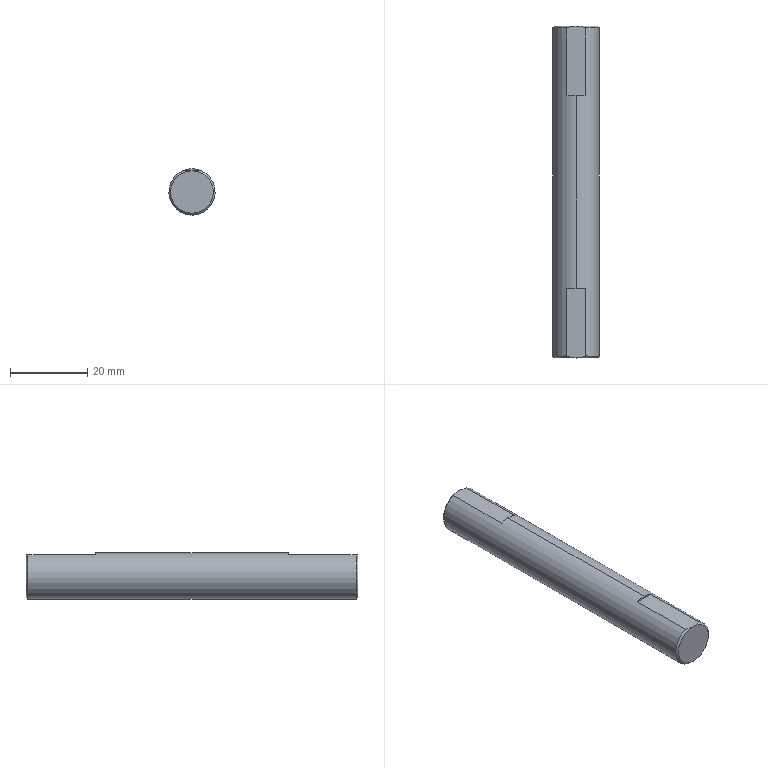Part | STEP file | ND25021-01-JDKM-18-GJ | 1 solid | 12 faces | box 12 x 86 x 12 mm | volume 9660 mm3 | plane 6 | cone 4 | cylinder 2 | commonest cylinder face diameters 12 x2
STEP:
#1=CARTESIAN_POINT('',(0.,0.,0.));
#2=DIRECTION('',(0.,0.,1.));
#3=DIRECTION('',(1.,0.,0.));
#4=AXIS2_PLACEMENT_3D('',#1,#2,#3);
#5=CARTESIAN_POINT('',(0.,-43.,-5.5));
#6=VERTEX_POINT('',#5);
#7=CARTESIAN_POINT('',(0.,-43.,5.5));
#8=VERTEX_POINT('',#7);
#9=CARTESIAN_POINT('',(0.,-43.,0.));
#10=DIRECTION('',(0.,-1.,0.));
#11=DIRECTION('',(0.,0.,1.));
#12=AXIS2_PLACEMENT_3D('',#9,#10,#11);
#13=CIRCLE('',#12,5.5);
#14=CARTESIAN_POINT('',(0.,-42.5,0.));
#15=DIRECTION('',(0.,1.,0.));
#16=DIRECTION('',(0.,0.,1.));
#17=AXIS2_PLACEMENT_3D('',#14,#15,#16);
#18=CONICAL_SURFACE('',#17,6.,0.7854);
#19=CARTESIAN_POINT('',(6.283,-0.5));
#20=DIRECTION('',(-1.,0.));
#21=VECTOR('',#20,1.);
#22=LINE('',#19,#21);
#23=(GEOMETRIC_REPRESENTATION_CONTEXT(2)PARAMETRIC_REPRESENTATION_CONTEXT()REPRESENTATION_CONTEXT('',''));
#24=DEFINITIONAL_REPRESENTATION('',(#22),#23);
#25=PCURVE('',#18,#24);
#26=CARTESIAN_POINT('',(0.,-43.,0.));
#27=DIRECTION('',(0.,1.,0.));
#28=DIRECTION('',(0.,0.,1.));
#29=AXIS2_PLACEMENT_3D('',#26,#27,#28);
#30=PLANE('',#29);
#31=CARTESIAN_POINT('',(5.5,0.));
#32=CARTESIAN_POINT('',(5.5,-9.526));
#33=CARTESIAN_POINT('',(-2.75,-4.763));
#34=CARTESIAN_POINT('',(-11.,0.));
#35=CARTESIAN_POINT('',(-2.75,4.763));
#36=CARTESIAN_POINT('',(5.5,9.526));
#37=CARTESIAN_POINT('',(5.5,0.));
#38=(BOUNDED_CURVE()B_SPLINE_CURVE(2,(#31,#32,#33,#34,#35,#36,#37),.UNSPECIFIED.,.T.,.F.)B_SPLINE_CURVE_WITH_KNOTS((1,2,2,2,2,1),(-2.094,0.,2.094,4.189,6.283,8.378),.UNSPECIFIED.)CURVE()GEOMETRIC_REPRESENTATION_ITEM()RATIONAL_B_SPLINE_CURVE((1.,0.5,1.,0.5,1.,0.5,1.))REPRESENTATION_ITEM(''));
#39=(GEOMETRIC_REPRESENTATION_CONTEXT(2)PARAMETRIC_REPRESENTATION_CONTEXT()REPRESENTATION_CONTEXT('',''));
#40=DEFINITIONAL_REPRESENTATION('',(#38),#39);
#41=PCURVE('',#30,#40);
#42=SURFACE_CURVE('',#13,(#25,#41),.PCURVE_S1.);
#43=EDGE_CURVE('',#6,#8,#42,.T.);
#44=ORIENTED_EDGE('',*,*,#43,.F.);
#45=CARTESIAN_POINT('',(0.,-42.5,-6.));
#46=VERTEX_POINT('',#45);
#47=CARTESIAN_POINT('',(0.,-42.5,-6.));
#48=DIRECTION('',(0.,0.7071,-0.7071));
#49=VECTOR('',#48,1.);
#50=LINE('',#47,#49);
#51=CARTESIAN_POINT('',(3.142,0.));
#52=DIRECTION('',(0.,1.));
#53=VECTOR('',#52,1.);
#54=LINE('',#51,#53);
#55=(GEOMETRIC_REPRESENTATION_CONTEXT(2)PARAMETRIC_REPRESENTATION_CONTEXT()REPRESENTATION_CONTEXT('',''));
#56=DEFINITIONAL_REPRESENTATION('',(#54),#55);
#57=PCURVE('',#18,#56);
#58=CARTESIAN_POINT('',(0.,-42.5,0.));
#59=DIRECTION('',(0.,1.,0.));
#60=DIRECTION('',(0.,0.,1.));
#61=AXIS2_PLACEMENT_3D('',#58,#59,#60);
#62=CONICAL_SURFACE('',#61,6.,0.7854);
#63=CARTESIAN_POINT('',(3.142,0.));
#64=DIRECTION('',(0.,1.));
#65=VECTOR('',#64,1.);
#66=LINE('',#63,#65);
#67=(GEOMETRIC_REPRESENTATION_CONTEXT(2)PARAMETRIC_REPRESENTATION_CONTEXT()REPRESENTATION_CONTEXT('',''));
#68=DEFINITIONAL_REPRESENTATION('',(#66),#67);
#69=PCURVE('',#62,#68);
#70=SURFACE_CURVE('',#50,(#57,#69),.PCURVE_S1.);
#71=EDGE_CURVE('',#6,#46,#70,.T.);
#72=ORIENTED_EDGE('',*,*,#71,.T.);
#73=CARTESIAN_POINT('',(2.398,-42.5,5.5));
#74=VERTEX_POINT('',#73);
#75=CARTESIAN_POINT('',(0.,-42.5,0.));
#76=DIRECTION('',(0.,1.,0.));
#77=DIRECTION('',(0.,0.,1.));
#78=AXIS2_PLACEMENT_3D('',#75,#76,#77);
#79=CIRCLE('',#78,6.);
#80=CARTESIAN_POINT('',(0.,0.));
#81=DIRECTION('',(1.,0.));
#82=VECTOR('',#81,1.);
#83=LINE('',#80,#82);
#84=(GEOMETRIC_REPRESENTATION_CONTEXT(2)PARAMETRIC_REPRESENTATION_CONTEXT()REPRESENTATION_CONTEXT('',''));
#85=DEFINITIONAL_REPRESENTATION('',(#83),#84);
#86=PCURVE('',#18,#85);
#87=CARTESIAN_POINT('',(0.,43.,0.));
#88=DIRECTION('',(0.,-1.,0.));
#89=DIRECTION('',(0.,0.,-1.));
#90=AXIS2_PLACEMENT_3D('',#87,#88,#89);
#91=CYLINDRICAL_SURFACE('',#90,6.);
#92=CARTESIAN_POINT('',(3.142,85.5));
#93=DIRECTION('',(-1.,0.));
#94=VECTOR('',#93,1.);
#95=LINE('',#92,#94);
#96=(GEOMETRIC_REPRESENTATION_CONTEXT(2)PARAMETRIC_REPRESENTATION_CONTEXT()REPRESENTATION_CONTEXT('',''));
#97=DEFINITIONAL_REPRESENTATION('',(#95),#96);
#98=PCURVE('',#91,#97);
#99=SURFACE_CURVE('',#79,(#86,#98),.PCURVE_S1.);
#100=EDGE_CURVE('',#74,#46,#99,.T.);
#101=ORIENTED_EDGE('',*,*,#100,.F.);
#102=CARTESIAN_POINT('',(0.,-43.,5.5));
#103=CARTESIAN_POINT('',(0.4145,-43.,5.5));
#104=CARTESIAN_POINT('',(0.8208,-42.953,5.5));
#105=CARTESIAN_POINT('',(1.62,-42.78,5.5));
#106=CARTESIAN_POINT('',(2.014,-42.653,5.5));
#107=CARTESIAN_POINT('',(2.398,-42.5,5.5));
#108=B_SPLINE_CURVE_WITH_KNOTS('',3,(#102,#103,#104,#105,#106,#107),.UNSPECIFIED.,.F.,.F.,(4,2,4),(0.,0.001225,0.00245),.UNSPECIFIED.);
#109=CARTESIAN_POINT('',(0.,-0.5));
#110=CARTESIAN_POINT('',(0.006852,-0.5));
#111=CARTESIAN_POINT('',(0.02053,-0.4992));
#112=CARTESIAN_POINT('',(0.04096,-0.4958));
#113=CARTESIAN_POINT('',(0.06128,-0.49));
#114=CARTESIAN_POINT('',(0.08148,-0.482));
#115=CARTESIAN_POINT('',(0.1015,-0.4719));
#116=CARTESIAN_POINT('',(0.1215,-0.4595));
#117=CARTESIAN_POINT('',(0.1412,-0.445));
#118=CARTESIAN_POINT('',(0.1608,-0.4285));
#119=CARTESIAN_POINT('',(0.1802,-0.4098));
#120=CARTESIAN_POINT('',(0.1994,-0.3892));
#121=CARTESIAN_POINT('',(0.2184,-0.3666));
#122=CARTESIAN_POINT('',(0.2372,-0.342));
#123=CARTESIAN_POINT('',(0.2557,-0.3155));
#124=CARTESIAN_POINT('',(0.274,-0.2871));
#125=CARTESIAN_POINT('',(0.2921,-0.257));
#126=CARTESIAN_POINT('',(0.31,-0.2251));
#127=CARTESIAN_POINT('',(0.3276,-0.1915));
#128=CARTESIAN_POINT('',(0.3449,-0.1563));
#129=CARTESIAN_POINT('',(0.3619,-0.1195));
#130=CARTESIAN_POINT('',(0.3786,-0.08115));
#131=CARTESIAN_POINT('',(0.395,-0.04138));
#132=CARTESIAN_POINT('',(0.4058,-0.01394));
#133=CARTESIAN_POINT('',(0.4111,0.));
#134=B_SPLINE_CURVE_WITH_KNOTS('',3,(#109,#110,#111,#112,#113,#114,#115,#116,#117,#118,#119,#120,#121,#122,#123,#124,#125,#126,#127,#128,#129,#130,#131,#132,#133),.UNSPECIFIED.,.F.,.F.,(4,1,1,1,1,1,1,1,1,1,1,1,1,1,1,1,1,1,1,1,1,1,4),(0.,0.0001114,0.0002228,0.0003341,0.0004455,0.0005569,0.0006683,0.0007797,0.0008911,0.001002,0.001114,0.001225,0.001337,0.001448,0.001559,0.001671,0.001782,0.001894,0.002005,0.002116,0.002228,0.002339,0.00245),.QUASI_UNIFORM_KNOTS.);
#135=(GEOMETRIC_REPRESENTATION_CONTEXT(2)PARAMETRIC_REPRESENTATION_CONTEXT()REPRESENTATION_CONTEXT('',''));
#136=DEFINITIONAL_REPRESENTATION('',(#134),#135);
#137=PCURVE('',#18,#136);
#138=CARTESIAN_POINT('',(-2.398,-25.,5.5));
#139=DIRECTION('',(0.,0.,-1.));
#140=DIRECTION('',(-1.,0.,0.));
#141=AXIS2_PLACEMENT_3D('',#138,#139,#140);
#142=PLANE('',#141);
#143=CARTESIAN_POINT('',(-2.398,-18.));
#144=CARTESIAN_POINT('',(-2.812,-18.));
#145=CARTESIAN_POINT('',(-3.219,-17.953));
#146=CARTESIAN_POINT('',(-4.018,-17.78));
#147=CARTESIAN_POINT('',(-4.412,-17.653));
#148=CARTESIAN_POINT('',(-4.796,-17.5));
#149=B_SPLINE_CURVE_WITH_KNOTS('',3,(#143,#144,#145,#146,#147,#148),.UNSPECIFIED.,.F.,.F.,(4,2,4),(0.,0.001225,0.00245),.UNSPECIFIED.);
#150=(GEOMETRIC_REPRESENTATION_CONTEXT(2)PARAMETRIC_REPRESENTATION_CONTEXT()REPRESENTATION_CONTEXT('',''));
#151=DEFINITIONAL_REPRESENTATION('',(#149),#150);
#152=PCURVE('',#142,#151);
#153=SURFACE_CURVE('',#108,(#137,#152),.PCURVE_S1.);
#154=EDGE_CURVE('',#8,#74,#153,.T.);
#155=ORIENTED_EDGE('',*,*,#154,.F.);
#156=EDGE_LOOP('',(#44,#72,#101,#155));
#157=FACE_BOUND('',#156,.T.);
#158=ADVANCED_FACE('',(#157),#18,.T.);
#159=CARTESIAN_POINT('',(0.,43.,-5.5));
#160=VERTEX_POINT('',#159);
#161=CARTESIAN_POINT('',(0.,43.,5.5));
#162=VERTEX_POINT('',#161);
#163=CARTESIAN_POINT('',(0.,43.,0.));
#164=DIRECTION('',(0.,1.,0.));
#165=DIRECTION('',(0.,0.,1.));
#166=AXIS2_PLACEMENT_3D('',#163,#164,#165);
#167=CIRCLE('',#166,5.5);
#168=CARTESIAN_POINT('',(0.,43.,0.));
#169=DIRECTION('',(0.,-1.,0.));
#170=DIRECTION('',(0.,0.,-1.));
#171=AXIS2_PLACEMENT_3D('',#168,#169,#170);
#172=CONICAL_SURFACE('',#171,5.5,0.7854);
#173=CARTESIAN_POINT('',(9.425,0.));
#174=DIRECTION('',(-1.,0.));
#175=VECTOR('',#174,1.);
#176=LINE('',#173,#175);
#177=(GEOMETRIC_REPRESENTATION_CONTEXT(2)PARAMETRIC_REPRESENTATION_CONTEXT()REPRESENTATION_CONTEXT('',''));
#178=DEFINITIONAL_REPRESENTATION('',(#176),#177);
#179=PCURVE('',#172,#178);
#180=CARTESIAN_POINT('',(0.,43.,0.));
#181=DIRECTION('',(0.,1.,0.));
#182=DIRECTION('',(0.,0.,1.));
#183=AXIS2_PLACEMENT_3D('',#180,#181,#182);
#184=PLANE('',#183);
#185=CARTESIAN_POINT('',(0.,0.));
#186=DIRECTION('',(1.,0.));
#187=AXIS2_PLACEMENT_2D('',#185,#186);
#188=CIRCLE('',#187,5.5);
#189=(GEOMETRIC_REPRESENTATION_CONTEXT(2)PARAMETRIC_REPRESENTATION_CONTEXT()REPRESENTATION_CONTEXT('',''));
#190=DEFINITIONAL_REPRESENTATION('',(#188),#189);
#191=PCURVE('',#184,#190);
#192=SURFACE_CURVE('',#167,(#179,#191),.PCURVE_S1.);
#193=EDGE_CURVE('',#160,#162,#192,.T.);
#194=ORIENTED_EDGE('',*,*,#193,.F.);
#195=CARTESIAN_POINT('',(0.,42.5,-6.));
#196=VERTEX_POINT('',#195);
#197=CARTESIAN_POINT('',(0.,43.,-5.5));
#198=DIRECTION('',(0.,-0.7071,-0.7071));
#199=VECTOR('',#198,1.);
#200=LINE('',#197,#199);
#201=CARTESIAN_POINT('',(6.283,0.));
#202=DIRECTION('',(0.,1.));
#203=VECTOR('',#202,1.);
#204=LINE('',#201,#203);
#205=(GEOMETRIC_REPRESENTATION_CONTEXT(2)PARAMETRIC_REPRESENTATION_CONTEXT()REPRESENTATION_CONTEXT('',''));
#206=DEFINITIONAL_REPRESENTATION('',(#204),#205);
#207=PCURVE('',#172,#206);
#208=CARTESIAN_POINT('',(0.,43.,0.));
#209=DIRECTION('',(0.,-1.,0.));
#210=DIRECTION('',(0.,0.,-1.));
#211=AXIS2_PLACEMENT_3D('',#208,#209,#210);
#212=CONICAL_SURFACE('',#211,5.5,0.7854);
#213=CARTESIAN_POINT('',(0.,0.));
#214=DIRECTION('',(0.,1.));
#215=VECTOR('',#214,1.);
#216=LINE('',#213,#215);
#217=(GEOMETRIC_REPRESENTATION_CONTEXT(2)PARAMETRIC_REPRESENTATION_CONTEXT()REPRESENTATION_CONTEXT('',''));
#218=DEFINITIONAL_REPRESENTATION('',(#216),#217);
#219=PCURVE('',#212,#218);
#220=SURFACE_CURVE('',#200,(#207,#219),.PCURVE_S1.);
#221=EDGE_CURVE('',#160,#196,#220,.T.);
#222=ORIENTED_EDGE('',*,*,#221,.T.);
#223=CARTESIAN_POINT('',(-2.398,42.5,5.5));
#224=VERTEX_POINT('',#223);
#225=CARTESIAN_POINT('',(0.,42.5,0.));
#226=DIRECTION('',(0.,-1.,0.));
#227=DIRECTION('',(0.,0.,1.));
#228=AXIS2_PLACEMENT_3D('',#225,#226,#227);
#229=CIRCLE('',#228,6.);
#230=CARTESIAN_POINT('',(3.142,0.5));
#231=DIRECTION('',(1.,0.));
#232=VECTOR('',#231,1.);
#233=LINE('',#230,#232);
#234=(GEOMETRIC_REPRESENTATION_CONTEXT(2)PARAMETRIC_REPRESENTATION_CONTEXT()REPRESENTATION_CONTEXT('',''));
#235=DEFINITIONAL_REPRESENTATION('',(#233),#234);
#236=PCURVE('',#172,#235);
#237=CARTESIAN_POINT('',(0.,43.,0.));
#238=DIRECTION('',(0.,-1.,0.));
#239=DIRECTION('',(0.,0.,-1.));
#240=AXIS2_PLACEMENT_3D('',#237,#238,#239);
#241=CYLINDRICAL_SURFACE('',#240,6.);
#242=CARTESIAN_POINT('',(3.142,0.5));
#243=DIRECTION('',(1.,0.));
#244=VECTOR('',#243,1.);
#245=LINE('',#242,#244);
#246=(GEOMETRIC_REPRESENTATION_CONTEXT(2)PARAMETRIC_REPRESENTATION_CONTEXT()REPRESENTATION_CONTEXT('',''));
#247=DEFINITIONAL_REPRESENTATION('',(#245),#246);
#248=PCURVE('',#241,#247);
#249=SURFACE_CURVE('',#229,(#236,#248),.PCURVE_S1.);
#250=EDGE_CURVE('',#224,#196,#249,.T.);
#251=ORIENTED_EDGE('',*,*,#250,.F.);
#252=CARTESIAN_POINT('',(0.,43.,5.5));
#253=CARTESIAN_POINT('',(-0.4145,43.,5.5));
#254=CARTESIAN_POINT('',(-0.8208,42.953,5.5));
#255=CARTESIAN_POINT('',(-1.62,42.78,5.5));
#256=CARTESIAN_POINT('',(-2.014,42.653,5.5));
#257=CARTESIAN_POINT('',(-2.398,42.5,5.5));
#258=B_SPLINE_CURVE_WITH_KNOTS('',3,(#252,#253,#254,#255,#256,#257),.UNSPECIFIED.,.F.,.F.,(4,2,4),(0.,0.001225,0.00245),.UNSPECIFIED.);
#259=CARTESIAN_POINT('',(3.142,0.));
#260=CARTESIAN_POINT('',(3.148,-0.000000092));
#261=CARTESIAN_POINT('',(3.162,0.0007776));
#262=CARTESIAN_POINT('',(3.183,0.004246));
#263=CARTESIAN_POINT('',(3.203,0.009984));
#264=CARTESIAN_POINT('',(3.223,0.01796));
#265=CARTESIAN_POINT('',(3.243,0.02814));
#266=CARTESIAN_POINT('',(3.263,0.04048));
#267=CARTESIAN_POINT('',(3.283,0.05496));
#268=CARTESIAN_POINT('',(3.302,0.07153));
#269=CARTESIAN_POINT('',(3.322,0.09015));
#270=CARTESIAN_POINT('',(3.341,0.1108));
#271=CARTESIAN_POINT('',(3.36,0.1334));
#272=CARTESIAN_POINT('',(3.379,0.158));
#273=CARTESIAN_POINT('',(3.397,0.1845));
#274=CARTESIAN_POINT('',(3.416,0.2129));
#275=CARTESIAN_POINT('',(3.434,0.243));
#276=CARTESIAN_POINT('',(3.452,0.2749));
#277=CARTESIAN_POINT('',(3.469,0.3085));
#278=CARTESIAN_POINT('',(3.486,0.3437));
#279=CARTESIAN_POINT('',(3.503,0.3805));
#280=CARTESIAN_POINT('',(3.52,0.4189));
#281=CARTESIAN_POINT('',(3.537,0.4586));
#282=CARTESIAN_POINT('',(3.547,0.4861));
#283=CARTESIAN_POINT('',(3.553,0.5));
#284=B_SPLINE_CURVE_WITH_KNOTS('',3,(#259,#260,#261,#262,#263,#264,#265,#266,#267,#268,#269,#270,#271,#272,#273,#274,#275,#276,#277,#278,#279,#280,#281,#282,#283),.UNSPECIFIED.,.F.,.F.,(4,1,1,1,1,1,1,1,1,1,1,1,1,1,1,1,1,1,1,1,1,1,4),(0.,0.0001114,0.0002228,0.0003341,0.0004455,0.0005569,0.0006683,0.0007797,0.0008911,0.001002,0.001114,0.001225,0.001337,0.001448,0.001559,0.001671,0.001782,0.001894,0.002005,0.002116,0.002228,0.002339,0.00245),.QUASI_UNIFORM_KNOTS.);
#285=(GEOMETRIC_REPRESENTATION_CONTEXT(2)PARAMETRIC_REPRESENTATION_CONTEXT()REPRESENTATION_CONTEXT('',''));
#286=DEFINITIONAL_REPRESENTATION('',(#284),#285);
#287=PCURVE('',#172,#286);
#288=CARTESIAN_POINT('',(-2.398,25.,5.5));
#289=DIRECTION('',(0.,0.,1.));
#290=DIRECTION('',(1.,0.,0.));
#291=AXIS2_PLACEMENT_3D('',#288,#289,#290);
#292=PLANE('',#291);
#293=CARTESIAN_POINT('',(2.398,18.));
#294=CARTESIAN_POINT('',(1.983,18.));
#295=CARTESIAN_POINT('',(1.577,17.953));
#296=CARTESIAN_POINT('',(0.7781,17.78));
#297=CARTESIAN_POINT('',(0.3837,17.653));
#298=CARTESIAN_POINT('',(0.,17.5));
#299=B_SPLINE_CURVE_WITH_KNOTS('',3,(#293,#294,#295,#296,#297,#298),.UNSPECIFIED.,.F.,.F.,(4,2,4),(0.,0.001225,0.00245),.UNSPECIFIED.);
#300=(GEOMETRIC_REPRESENTATION_CONTEXT(2)PARAMETRIC_REPRESENTATION_CONTEXT()REPRESENTATION_CONTEXT('',''));
#301=DEFINITIONAL_REPRESENTATION('',(#299),#300);
#302=PCURVE('',#292,#301);
#303=SURFACE_CURVE('',#258,(#287,#302),.PCURVE_S1.);
#304=EDGE_CURVE('',#162,#224,#303,.T.);
#305=ORIENTED_EDGE('',*,*,#304,.F.);
#306=EDGE_LOOP('',(#194,#222,#251,#305));
#307=FACE_BOUND('',#306,.T.);
#308=ADVANCED_FACE('',(#307),#172,.T.);
#309=CARTESIAN_POINT('',(0.,25.,6.));
#310=VERTEX_POINT('',#309);
#311=CARTESIAN_POINT('',(2.398,25.,5.5));
#312=VERTEX_POINT('',#311);
#313=CARTESIAN_POINT('',(0.,25.,0.));
#314=DIRECTION('',(0.,1.,0.));
#315=DIRECTION('',(0.,0.,1.));
#316=AXIS2_PLACEMENT_3D('',#313,#314,#315);
#317=CIRCLE('',#316,6.);
#318=CARTESIAN_POINT('',(3.142,18.));
#319=DIRECTION('',(-1.,0.));
#320=VECTOR('',#319,1.);
#321=LINE('',#318,#320);
#322=(GEOMETRIC_REPRESENTATION_CONTEXT(2)PARAMETRIC_REPRESENTATION_CONTEXT()REPRESENTATION_CONTEXT('',''));
#323=DEFINITIONAL_REPRESENTATION('',(#321),#322);
#324=PCURVE('',#91,#323);
#325=CARTESIAN_POINT('',(0.,25.,0.));
#326=DIRECTION('',(0.,1.,0.));
#327=DIRECTION('',(0.,0.,-1.));
#328=AXIS2_PLACEMENT_3D('',#325,#326,#327);
#329=PLANE('',#328);
#330=CARTESIAN_POINT('',(0.,0.));
#331=DIRECTION('',(-1.,0.));
#332=AXIS2_PLACEMENT_2D('',#330,#331);
#333=CIRCLE('',#332,6.);
#334=(GEOMETRIC_REPRESENTATION_CONTEXT(2)PARAMETRIC_REPRESENTATION_CONTEXT()REPRESENTATION_CONTEXT('',''));
#335=DEFINITIONAL_REPRESENTATION('',(#333),#334);
#336=PCURVE('',#329,#335);
#337=SURFACE_CURVE('',#317,(#324,#336),.PCURVE_S1.);
#338=EDGE_CURVE('',#310,#312,#337,.T.);
#339=ORIENTED_EDGE('',*,*,#338,.F.);
#340=CARTESIAN_POINT('',(0.,-25.,6.));
#341=VERTEX_POINT('',#340);
#342=CARTESIAN_POINT('',(0.,43.,6.));
#343=DIRECTION('',(0.,-1.,0.));
#344=VECTOR('',#343,1.);
#345=LINE('',#342,#344);
#346=CARTESIAN_POINT('',(3.142,0.));
#347=DIRECTION('',(0.,1.));
#348=VECTOR('',#347,1.);
#349=LINE('',#346,#348);
#350=(GEOMETRIC_REPRESENTATION_CONTEXT(2)PARAMETRIC_REPRESENTATION_CONTEXT()REPRESENTATION_CONTEXT('',''));
#351=DEFINITIONAL_REPRESENTATION('',(#349),#350);
#352=PCURVE('',#91,#351);
#353=CARTESIAN_POINT('',(3.142,0.));
#354=DIRECTION('',(0.,1.));
#355=VECTOR('',#354,1.);
#356=LINE('',#353,#355);
#357=(GEOMETRIC_REPRESENTATION_CONTEXT(2)PARAMETRIC_REPRESENTATION_CONTEXT()REPRESENTATION_CONTEXT('',''));
#358=DEFINITIONAL_REPRESENTATION('',(#356),#357);
#359=PCURVE('',#241,#358);
#360=SURFACE_CURVE('',#345,(#352,#359),.PCURVE_S1.);
#361=EDGE_CURVE('',#310,#341,#360,.T.);
#362=ORIENTED_EDGE('',*,*,#361,.T.);
#363=CARTESIAN_POINT('',(2.398,-25.,5.5));
#364=VERTEX_POINT('',#363);
#365=CARTESIAN_POINT('',(0.,-25.,0.));
#366=DIRECTION('',(0.,-1.,0.));
#367=DIRECTION('',(0.,0.,-1.));
#368=AXIS2_PLACEMENT_3D('',#365,#366,#367);
#369=CIRCLE('',#368,6.);
#370=CARTESIAN_POINT('',(0.,68.));
#371=DIRECTION('',(1.,0.));
#372=VECTOR('',#371,1.);
#373=LINE('',#370,#372);
#374=(GEOMETRIC_REPRESENTATION_CONTEXT(2)PARAMETRIC_REPRESENTATION_CONTEXT()REPRESENTATION_CONTEXT('',''));
#375=DEFINITIONAL_REPRESENTATION('',(#373),#374);
#376=PCURVE('',#91,#375);
#377=CARTESIAN_POINT('',(0.,-25.,0.));
#378=DIRECTION('',(0.,-1.,0.));
#379=DIRECTION('',(0.,0.,-1.));
#380=AXIS2_PLACEMENT_3D('',#377,#378,#379);
#381=PLANE('',#380);
#382=CARTESIAN_POINT('',(0.,0.));
#383=DIRECTION('',(1.,0.));
#384=AXIS2_PLACEMENT_2D('',#382,#383);
#385=CIRCLE('',#384,6.);
#386=(GEOMETRIC_REPRESENTATION_CONTEXT(2)PARAMETRIC_REPRESENTATION_CONTEXT()REPRESENTATION_CONTEXT('',''));
#387=DEFINITIONAL_REPRESENTATION('',(#385),#386);
#388=PCURVE('',#381,#387);
#389=SURFACE_CURVE('',#369,(#376,#388),.PCURVE_S1.);
#390=EDGE_CURVE('',#364,#341,#389,.T.);
#391=ORIENTED_EDGE('',*,*,#390,.F.);
#392=CARTESIAN_POINT('',(2.398,-25.,5.5));
#393=DIRECTION('',(0.,-1.,0.));
#394=VECTOR('',#393,1.);
#395=LINE('',#392,#394);
#396=CARTESIAN_POINT('',(2.73,68.));
#397=DIRECTION('',(0.,1.));
#398=VECTOR('',#397,1.);
#399=LINE('',#396,#398);
#400=(GEOMETRIC_REPRESENTATION_CONTEXT(2)PARAMETRIC_REPRESENTATION_CONTEXT()REPRESENTATION_CONTEXT('',''));
#401=DEFINITIONAL_REPRESENTATION('',(#399),#400);
#402=PCURVE('',#91,#401);
#403=CARTESIAN_POINT('',(-4.796,0.));
#404=DIRECTION('',(0.,-1.));
#405=VECTOR('',#404,1.);
#406=LINE('',#403,#405);
#407=(GEOMETRIC_REPRESENTATION_CONTEXT(2)PARAMETRIC_REPRESENTATION_CONTEXT()REPRESENTATION_CONTEXT('',''));
#408=DEFINITIONAL_REPRESENTATION('',(#406),#407);
#409=PCURVE('',#142,#408);
#410=SURFACE_CURVE('',#395,(#402,#409),.PCURVE_S1.);
#411=EDGE_CURVE('',#364,#74,#410,.T.);
#412=ORIENTED_EDGE('',*,*,#411,.T.);
#413=ORIENTED_EDGE('',*,*,#100,.T.);
#414=CARTESIAN_POINT('',(0.,43.,-6.));
#415=DIRECTION('',(0.,-1.,0.));
#416=VECTOR('',#415,1.);
#417=LINE('',#414,#416);
#418=CARTESIAN_POINT('',(0.,0.));
#419=DIRECTION('',(0.,1.));
#420=VECTOR('',#419,1.);
#421=LINE('',#418,#420);
#422=(GEOMETRIC_REPRESENTATION_CONTEXT(2)PARAMETRIC_REPRESENTATION_CONTEXT()REPRESENTATION_CONTEXT('',''));
#423=DEFINITIONAL_REPRESENTATION('',(#421),#422);
#424=PCURVE('',#91,#423);
#425=CARTESIAN_POINT('',(6.283,0.));
#426=DIRECTION('',(0.,1.));
#427=VECTOR('',#426,1.);
#428=LINE('',#425,#427);
#429=(GEOMETRIC_REPRESENTATION_CONTEXT(2)PARAMETRIC_REPRESENTATION_CONTEXT()REPRESENTATION_CONTEXT('',''));
#430=DEFINITIONAL_REPRESENTATION('',(#428),#429);
#431=PCURVE('',#241,#430);
#432=SURFACE_CURVE('',#417,(#424,#431),.PCURVE_S1.);
#433=EDGE_CURVE('',#196,#46,#432,.T.);
#434=ORIENTED_EDGE('',*,*,#433,.F.);
#435=CARTESIAN_POINT('',(2.398,42.5,5.5));
#436=VERTEX_POINT('',#435);
#437=CARTESIAN_POINT('',(0.,42.5,0.));
#438=DIRECTION('',(0.,-1.,0.));
#439=DIRECTION('',(0.,0.,1.));
#440=AXIS2_PLACEMENT_3D('',#437,#438,#439);
#441=CIRCLE('',#440,6.);
#442=CARTESIAN_POINT('',(-3.142,0.5));
#443=DIRECTION('',(1.,0.));
#444=VECTOR('',#443,1.);
#445=LINE('',#442,#444);
#446=(GEOMETRIC_REPRESENTATION_CONTEXT(2)PARAMETRIC_REPRESENTATION_CONTEXT()REPRESENTATION_CONTEXT('',''));
#447=DEFINITIONAL_REPRESENTATION('',(#445),#446);
#448=PCURVE('',#91,#447);
#449=CARTESIAN_POINT('',(-3.142,0.5));
#450=DIRECTION('',(1.,0.));
#451=VECTOR('',#450,1.);
#452=LINE('',#449,#451);
#453=(GEOMETRIC_REPRESENTATION_CONTEXT(2)PARAMETRIC_REPRESENTATION_CONTEXT()REPRESENTATION_CONTEXT('',''));
#454=DEFINITIONAL_REPRESENTATION('',(#452),#453);
#455=PCURVE('',#212,#454);
#456=SURFACE_CURVE('',#441,(#448,#455),.PCURVE_S1.);
#457=EDGE_CURVE('',#196,#436,#456,.T.);
#458=ORIENTED_EDGE('',*,*,#457,.T.);
#459=CARTESIAN_POINT('',(2.398,25.,5.5));
#460=DIRECTION('',(0.,1.,0.));
#461=VECTOR('',#460,1.);
#462=LINE('',#459,#461);
#463=CARTESIAN_POINT('',(2.73,18.));
#464=DIRECTION('',(0.,-1.));
#465=VECTOR('',#464,1.);
#466=LINE('',#463,#465);
#467=(GEOMETRIC_REPRESENTATION_CONTEXT(2)PARAMETRIC_REPRESENTATION_CONTEXT()REPRESENTATION_CONTEXT('',''));
#468=DEFINITIONAL_REPRESENTATION('',(#466),#467);
#469=PCURVE('',#91,#468);
#470=CARTESIAN_POINT('',(4.796,0.));
#471=DIRECTION('',(0.,1.));
#472=VECTOR('',#471,1.);
#473=LINE('',#470,#472);
#474=(GEOMETRIC_REPRESENTATION_CONTEXT(2)PARAMETRIC_REPRESENTATION_CONTEXT()REPRESENTATION_CONTEXT('',''));
#475=DEFINITIONAL_REPRESENTATION('',(#473),#474);
#476=PCURVE('',#292,#475);
#477=SURFACE_CURVE('',#462,(#469,#476),.PCURVE_S1.);
#478=EDGE_CURVE('',#312,#436,#477,.T.);
#479=ORIENTED_EDGE('',*,*,#478,.F.);
#480=EDGE_LOOP('',(#339,#362,#391,#412,#413,#434,#458,#479));
#481=FACE_BOUND('',#480,.T.);
#482=ADVANCED_FACE('',(#481),#91,.T.);
#483=ORIENTED_EDGE('',*,*,#361,.F.);
#484=CARTESIAN_POINT('',(-2.398,25.,5.5));
#485=VERTEX_POINT('',#484);
#486=CARTESIAN_POINT('',(0.,25.,0.));
#487=DIRECTION('',(0.,1.,0.));
#488=DIRECTION('',(0.,0.,1.));
#489=AXIS2_PLACEMENT_3D('',#486,#487,#488);
#490=CIRCLE('',#489,6.);
#491=CARTESIAN_POINT('',(9.425,18.));
#492=DIRECTION('',(-1.,0.));
#493=VECTOR('',#492,1.);
#494=LINE('',#491,#493);
#495=(GEOMETRIC_REPRESENTATION_CONTEXT(2)PARAMETRIC_REPRESENTATION_CONTEXT()REPRESENTATION_CONTEXT('',''));
#496=DEFINITIONAL_REPRESENTATION('',(#494),#495);
#497=PCURVE('',#241,#496);
#498=CARTESIAN_POINT('',(0.,0.));
#499=DIRECTION('',(-1.,0.));
#500=AXIS2_PLACEMENT_2D('',#498,#499);
#501=CIRCLE('',#500,6.);
#502=(GEOMETRIC_REPRESENTATION_CONTEXT(2)PARAMETRIC_REPRESENTATION_CONTEXT()REPRESENTATION_CONTEXT('',''));
#503=DEFINITIONAL_REPRESENTATION('',(#501),#502);
#504=PCURVE('',#329,#503);
#505=SURFACE_CURVE('',#490,(#497,#504),.PCURVE_S1.);
#506=EDGE_CURVE('',#485,#310,#505,.T.);
#507=ORIENTED_EDGE('',*,*,#506,.F.);
#508=CARTESIAN_POINT('',(-2.398,25.,5.5));
#509=DIRECTION('',(0.,1.,0.));
#510=VECTOR('',#509,1.);
#511=LINE('',#508,#510);
#512=CARTESIAN_POINT('',(3.553,18.));
#513=DIRECTION('',(0.,-1.));
#514=VECTOR('',#513,1.);
#515=LINE('',#512,#514);
#516=(GEOMETRIC_REPRESENTATION_CONTEXT(2)PARAMETRIC_REPRESENTATION_CONTEXT()REPRESENTATION_CONTEXT('',''));
#517=DEFINITIONAL_REPRESENTATION('',(#515),#516);
#518=PCURVE('',#241,#517);
#519=CARTESIAN_POINT('',(0.,0.));
#520=DIRECTION('',(0.,1.));
#521=VECTOR('',#520,1.);
#522=LINE('',#519,#521);
#523=(GEOMETRIC_REPRESENTATION_CONTEXT(2)PARAMETRIC_REPRESENTATION_CONTEXT()REPRESENTATION_CONTEXT('',''));
#524=DEFINITIONAL_REPRESENTATION('',(#522),#523);
#525=PCURVE('',#292,#524);
#526=SURFACE_CURVE('',#511,(#518,#525),.PCURVE_S1.);
#527=EDGE_CURVE('',#485,#224,#526,.T.);
#528=ORIENTED_EDGE('',*,*,#527,.T.);
#529=ORIENTED_EDGE('',*,*,#250,.T.);
#530=ORIENTED_EDGE('',*,*,#433,.T.);
#531=CARTESIAN_POINT('',(-2.398,-42.5,5.5));
#532=VERTEX_POINT('',#531);
#533=CARTESIAN_POINT('',(0.,-42.5,0.));
#534=DIRECTION('',(0.,1.,0.));
#535=DIRECTION('',(0.,0.,1.));
#536=AXIS2_PLACEMENT_3D('',#533,#534,#535);
#537=CIRCLE('',#536,6.);
#538=CARTESIAN_POINT('',(9.425,85.5));
#539=DIRECTION('',(-1.,0.));
#540=VECTOR('',#539,1.);
#541=LINE('',#538,#540);
#542=(GEOMETRIC_REPRESENTATION_CONTEXT(2)PARAMETRIC_REPRESENTATION_CONTEXT()REPRESENTATION_CONTEXT('',''));
#543=DEFINITIONAL_REPRESENTATION('',(#541),#542);
#544=PCURVE('',#241,#543);
#545=CARTESIAN_POINT('',(0.,0.));
#546=DIRECTION('',(1.,0.));
#547=VECTOR('',#546,1.);
#548=LINE('',#545,#547);
#549=(GEOMETRIC_REPRESENTATION_CONTEXT(2)PARAMETRIC_REPRESENTATION_CONTEXT()REPRESENTATION_CONTEXT('',''));
#550=DEFINITIONAL_REPRESENTATION('',(#548),#549);
#551=PCURVE('',#62,#550);
#552=SURFACE_CURVE('',#537,(#544,#551),.PCURVE_S1.);
#553=EDGE_CURVE('',#46,#532,#552,.T.);
#554=ORIENTED_EDGE('',*,*,#553,.T.);
#555=CARTESIAN_POINT('',(-2.398,-25.,5.5));
#556=VERTEX_POINT('',#555);
#557=CARTESIAN_POINT('',(-2.398,-25.,5.5));
#558=DIRECTION('',(0.,-1.,0.));
#559=VECTOR('',#558,1.);
#560=LINE('',#557,#559);
#561=CARTESIAN_POINT('',(3.553,68.));
#562=DIRECTION('',(0.,1.));
#563=VECTOR('',#562,1.);
#564=LINE('',#561,#563);
#565=(GEOMETRIC_REPRESENTATION_CONTEXT(2)PARAMETRIC_REPRESENTATION_CONTEXT()REPRESENTATION_CONTEXT('',''));
#566=DEFINITIONAL_REPRESENTATION('',(#564),#565);
#567=PCURVE('',#241,#566);
#568=CARTESIAN_POINT('',(0.,0.));
#569=DIRECTION('',(0.,-1.));
#570=VECTOR('',#569,1.);
#571=LINE('',#568,#570);
#572=(GEOMETRIC_REPRESENTATION_CONTEXT(2)PARAMETRIC_REPRESENTATION_CONTEXT()REPRESENTATION_CONTEXT('',''));
#573=DEFINITIONAL_REPRESENTATION('',(#571),#572);
#574=PCURVE('',#142,#573);
#575=SURFACE_CURVE('',#560,(#567,#574),.PCURVE_S1.);
#576=EDGE_CURVE('',#556,#532,#575,.T.);
#577=ORIENTED_EDGE('',*,*,#576,.F.);
#578=CARTESIAN_POINT('',(0.,-25.,0.));
#579=DIRECTION('',(0.,-1.,0.));
#580=DIRECTION('',(0.,0.,-1.));
#581=AXIS2_PLACEMENT_3D('',#578,#579,#580);
#582=CIRCLE('',#581,6.);
#583=CARTESIAN_POINT('',(0.,68.));
#584=DIRECTION('',(1.,0.));
#585=VECTOR('',#584,1.);
#586=LINE('',#583,#585);
#587=(GEOMETRIC_REPRESENTATION_CONTEXT(2)PARAMETRIC_REPRESENTATION_CONTEXT()REPRESENTATION_CONTEXT('',''));
#588=DEFINITIONAL_REPRESENTATION('',(#586),#587);
#589=PCURVE('',#241,#588);
#590=CARTESIAN_POINT('',(0.,0.));
#591=DIRECTION('',(1.,0.));
#592=AXIS2_PLACEMENT_2D('',#590,#591);
#593=CIRCLE('',#592,6.);
#594=(GEOMETRIC_REPRESENTATION_CONTEXT(2)PARAMETRIC_REPRESENTATION_CONTEXT()REPRESENTATION_CONTEXT('',''));
#595=DEFINITIONAL_REPRESENTATION('',(#593),#594);
#596=PCURVE('',#381,#595);
#597=SURFACE_CURVE('',#582,(#589,#596),.PCURVE_S1.);
#598=EDGE_CURVE('',#341,#556,#597,.T.);
#599=ORIENTED_EDGE('',*,*,#598,.F.);
#600=EDGE_LOOP('',(#483,#507,#528,#529,#530,#554,#577,#599));
#601=FACE_BOUND('',#600,.T.);
#602=ADVANCED_FACE('',(#601),#241,.T.);
#603=CARTESIAN_POINT('',(0.,43.,0.));
#604=DIRECTION('',(0.,1.,0.));
#605=DIRECTION('',(0.,0.,1.));
#606=AXIS2_PLACEMENT_3D('',#603,#604,#605);
#607=CIRCLE('',#606,5.5);
#608=CARTESIAN_POINT('',(0.,0.));
#609=DIRECTION('',(1.,0.));
#610=AXIS2_PLACEMENT_2D('',#608,#609);
#611=CIRCLE('',#610,5.5);
#612=(GEOMETRIC_REPRESENTATION_CONTEXT(2)PARAMETRIC_REPRESENTATION_CONTEXT()REPRESENTATION_CONTEXT('',''));
#613=DEFINITIONAL_REPRESENTATION('',(#611),#612);
#614=PCURVE('',#184,#613);
#615=CARTESIAN_POINT('',(3.142,0.));
#616=DIRECTION('',(-1.,0.));
#617=VECTOR('',#616,1.);
#618=LINE('',#615,#617);
#619=(GEOMETRIC_REPRESENTATION_CONTEXT(2)PARAMETRIC_REPRESENTATION_CONTEXT()REPRESENTATION_CONTEXT('',''));
#620=DEFINITIONAL_REPRESENTATION('',(#618),#619);
#621=PCURVE('',#212,#620);
#622=SURFACE_CURVE('',#607,(#614,#621),.PCURVE_S1.);
#623=EDGE_CURVE('',#162,#160,#622,.T.);
#624=ORIENTED_EDGE('',*,*,#623,.T.);
#625=ORIENTED_EDGE('',*,*,#193,.T.);
#626=EDGE_LOOP('',(#624,#625));
#627=FACE_BOUND('',#626,.T.);
#628=ADVANCED_FACE('',(#627),#184,.T.);
#629=CARTESIAN_POINT('',(0.,-43.,0.));
#630=DIRECTION('',(0.,-1.,0.));
#631=DIRECTION('',(0.,0.,1.));
#632=AXIS2_PLACEMENT_3D('',#629,#630,#631);
#633=CIRCLE('',#632,5.5);
#634=CARTESIAN_POINT('',(5.5,0.));
#635=CARTESIAN_POINT('',(5.5,-9.526));
#636=CARTESIAN_POINT('',(-2.75,-4.763));
#637=CARTESIAN_POINT('',(-11.,0.));
#638=CARTESIAN_POINT('',(-2.75,4.763));
#639=CARTESIAN_POINT('',(5.5,9.526));
#640=CARTESIAN_POINT('',(5.5,0.));
#641=(BOUNDED_CURVE()B_SPLINE_CURVE(2,(#634,#635,#636,#637,#638,#639,#640),.UNSPECIFIED.,.T.,.F.)B_SPLINE_CURVE_WITH_KNOTS((1,2,2,2,2,1),(-2.094,0.,2.094,4.189,6.283,8.378),.UNSPECIFIED.)CURVE()GEOMETRIC_REPRESENTATION_ITEM()RATIONAL_B_SPLINE_CURVE((1.,0.5,1.,0.5,1.,0.5,1.))REPRESENTATION_ITEM(''));
#642=(GEOMETRIC_REPRESENTATION_CONTEXT(2)PARAMETRIC_REPRESENTATION_CONTEXT()REPRESENTATION_CONTEXT('',''));
#643=DEFINITIONAL_REPRESENTATION('',(#641),#642);
#644=PCURVE('',#30,#643);
#645=CARTESIAN_POINT('',(6.283,-0.5));
#646=DIRECTION('',(-1.,0.));
#647=VECTOR('',#646,1.);
#648=LINE('',#645,#647);
#649=(GEOMETRIC_REPRESENTATION_CONTEXT(2)PARAMETRIC_REPRESENTATION_CONTEXT()REPRESENTATION_CONTEXT('',''));
#650=DEFINITIONAL_REPRESENTATION('',(#648),#649);
#651=PCURVE('',#62,#650);
#652=SURFACE_CURVE('',#633,(#644,#651),.PCURVE_S1.);
#653=EDGE_CURVE('',#8,#6,#652,.T.);
#654=ORIENTED_EDGE('',*,*,#653,.T.);
#655=ORIENTED_EDGE('',*,*,#43,.T.);
#656=EDGE_LOOP('',(#654,#655));
#657=FACE_BOUND('',#656,.T.);
#658=ADVANCED_FACE('',(#657),#30,.F.);
#659=CARTESIAN_POINT('',(-2.398,-25.,5.5));
#660=DIRECTION('',(1.,0.,0.));
#661=VECTOR('',#660,1.);
#662=LINE('',#659,#661);
#663=CARTESIAN_POINT('',(-5.5,-2.398));
#664=DIRECTION('',(0.,1.));
#665=VECTOR('',#664,1.);
#666=LINE('',#663,#665);
#667=(GEOMETRIC_REPRESENTATION_CONTEXT(2)PARAMETRIC_REPRESENTATION_CONTEXT()REPRESENTATION_CONTEXT('',''));
#668=DEFINITIONAL_REPRESENTATION('',(#666),#667);
#669=PCURVE('',#381,#668);
#670=CARTESIAN_POINT('',(0.,0.));
#671=DIRECTION('',(-1.,0.));
#672=VECTOR('',#671,1.);
#673=LINE('',#670,#672);
#674=(GEOMETRIC_REPRESENTATION_CONTEXT(2)PARAMETRIC_REPRESENTATION_CONTEXT()REPRESENTATION_CONTEXT('',''));
#675=DEFINITIONAL_REPRESENTATION('',(#673),#674);
#676=PCURVE('',#142,#675);
#677=SURFACE_CURVE('',#662,(#669,#676),.PCURVE_S1.);
#678=EDGE_CURVE('',#556,#364,#677,.T.);
#679=ORIENTED_EDGE('',*,*,#678,.T.);
#680=ORIENTED_EDGE('',*,*,#390,.T.);
#681=ORIENTED_EDGE('',*,*,#598,.T.);
#682=EDGE_LOOP('',(#679,#680,#681));
#683=FACE_BOUND('',#682,.T.);
#684=ADVANCED_FACE('',(#683),#381,.T.);
#685=ORIENTED_EDGE('',*,*,#576,.T.);
#686=CARTESIAN_POINT('',(-2.398,-42.5,5.5));
#687=CARTESIAN_POINT('',(-1.628,-42.808,5.5));
#688=CARTESIAN_POINT('',(-0.8341,-43.,5.5));
#689=CARTESIAN_POINT('',(0.,-43.,5.5));
#690=B_SPLINE_CURVE_WITH_KNOTS('',3,(#686,#687,#688,#689),.UNSPECIFIED.,.F.,.F.,(4,4),(0.,0.002449),.PIECEWISE_BEZIER_KNOTS.);
#691=CARTESIAN_POINT('',(0.,-17.5));
#692=CARTESIAN_POINT('',(-0.7699,-17.808));
#693=CARTESIAN_POINT('',(-1.564,-18.));
#694=CARTESIAN_POINT('',(-2.398,-18.));
#695=B_SPLINE_CURVE_WITH_KNOTS('',3,(#691,#692,#693,#694),.UNSPECIFIED.,.F.,.F.,(4,4),(0.,0.002449),.PIECEWISE_BEZIER_KNOTS.);
#696=(GEOMETRIC_REPRESENTATION_CONTEXT(2)PARAMETRIC_REPRESENTATION_CONTEXT()REPRESENTATION_CONTEXT('',''));
#697=DEFINITIONAL_REPRESENTATION('',(#695),#696);
#698=PCURVE('',#142,#697);
#699=CARTESIAN_POINT('',(5.872,0.));
#700=CARTESIAN_POINT('',(5.877,-0.01399));
#701=CARTESIAN_POINT('',(5.888,-0.04148));
#702=CARTESIAN_POINT('',(5.905,-0.08126));
#703=CARTESIAN_POINT('',(5.921,-0.1195));
#704=CARTESIAN_POINT('',(5.938,-0.1562));
#705=CARTESIAN_POINT('',(5.956,-0.1913));
#706=CARTESIAN_POINT('',(5.973,-0.2248));
#707=CARTESIAN_POINT('',(5.991,-0.2566));
#708=CARTESIAN_POINT('',(6.009,-0.2866));
#709=CARTESIAN_POINT('',(6.027,-0.3148));
#710=CARTESIAN_POINT('',(6.046,-0.3413));
#711=CARTESIAN_POINT('',(6.064,-0.3658));
#712=CARTESIAN_POINT('',(6.083,-0.3885));
#713=CARTESIAN_POINT('',(6.102,-0.4092));
#714=CARTESIAN_POINT('',(6.122,-0.4279));
#715=CARTESIAN_POINT('',(6.141,-0.4446));
#716=CARTESIAN_POINT('',(6.161,-0.4591));
#717=CARTESIAN_POINT('',(6.181,-0.4716));
#718=CARTESIAN_POINT('',(6.201,-0.4818));
#719=CARTESIAN_POINT('',(6.222,-0.4899));
#720=CARTESIAN_POINT('',(6.242,-0.4957));
#721=CARTESIAN_POINT('',(6.263,-0.4992));
#722=CARTESIAN_POINT('',(6.276,-0.5));
#723=CARTESIAN_POINT('',(6.283,-0.5));
#724=B_SPLINE_CURVE_WITH_KNOTS('',3,(#699,#700,#701,#702,#703,#704,#705,#706,#707,#708,#709,#710,#711,#712,#713,#714,#715,#716,#717,#718,#719,#720,#721,#722,#723),.UNSPECIFIED.,.F.,.F.,(4,1,1,1,1,1,1,1,1,1,1,1,1,1,1,1,1,1,1,1,1,1,4),(0.,0.0001113,0.0002227,0.000334,0.0004454,0.0005567,0.000668,0.0007794,0.0008907,0.001002,0.001113,0.001225,0.001336,0.001447,0.001559,0.00167,0.001781,0.001893,0.002004,0.002115,0.002227,0.002338,0.002449),.QUASI_UNIFORM_KNOTS.);
#725=(GEOMETRIC_REPRESENTATION_CONTEXT(2)PARAMETRIC_REPRESENTATION_CONTEXT()REPRESENTATION_CONTEXT('',''));
#726=DEFINITIONAL_REPRESENTATION('',(#724),#725);
#727=PCURVE('',#62,#726);
#728=SURFACE_CURVE('',#690,(#698,#727),.PCURVE_S1.);
#729=EDGE_CURVE('',#532,#8,#728,.T.);
#730=ORIENTED_EDGE('',*,*,#729,.T.);
#731=ORIENTED_EDGE('',*,*,#154,.T.);
#732=ORIENTED_EDGE('',*,*,#411,.F.);
#733=ORIENTED_EDGE('',*,*,#678,.F.);
#734=EDGE_LOOP('',(#685,#730,#731,#732,#733));
#735=FACE_BOUND('',#734,.T.);
#736=ADVANCED_FACE('',(#735),#142,.F.);
#737=ORIENTED_EDGE('',*,*,#506,.T.);
#738=ORIENTED_EDGE('',*,*,#338,.T.);
#739=CARTESIAN_POINT('',(-2.398,25.,5.5));
#740=DIRECTION('',(1.,0.,0.));
#741=VECTOR('',#740,1.);
#742=LINE('',#739,#741);
#743=CARTESIAN_POINT('',(-5.5,2.398));
#744=DIRECTION('',(0.,-1.));
#745=VECTOR('',#744,1.);
#746=LINE('',#743,#745);
#747=(GEOMETRIC_REPRESENTATION_CONTEXT(2)PARAMETRIC_REPRESENTATION_CONTEXT()REPRESENTATION_CONTEXT('',''));
#748=DEFINITIONAL_REPRESENTATION('',(#746),#747);
#749=PCURVE('',#329,#748);
#750=CARTESIAN_POINT('',(0.,0.));
#751=DIRECTION('',(1.,0.));
#752=VECTOR('',#751,1.);
#753=LINE('',#750,#752);
#754=(GEOMETRIC_REPRESENTATION_CONTEXT(2)PARAMETRIC_REPRESENTATION_CONTEXT()REPRESENTATION_CONTEXT('',''));
#755=DEFINITIONAL_REPRESENTATION('',(#753),#754);
#756=PCURVE('',#292,#755);
#757=SURFACE_CURVE('',#742,(#749,#756),.PCURVE_S1.);
#758=EDGE_CURVE('',#485,#312,#757,.T.);
#759=ORIENTED_EDGE('',*,*,#758,.F.);
#760=EDGE_LOOP('',(#737,#738,#759));
#761=FACE_BOUND('',#760,.T.);
#762=ADVANCED_FACE('',(#761),#329,.T.);
#763=CARTESIAN_POINT('',(2.398,42.5,5.5));
#764=CARTESIAN_POINT('',(1.628,42.808,5.5));
#765=CARTESIAN_POINT('',(0.8341,43.,5.5));
#766=CARTESIAN_POINT('',(0.,43.,5.5));
#767=B_SPLINE_CURVE_WITH_KNOTS('',3,(#763,#764,#765,#766),.UNSPECIFIED.,.F.,.F.,(4,4),(0.,0.002449),.PIECEWISE_BEZIER_KNOTS.);
#768=CARTESIAN_POINT('',(4.796,17.5));
#769=CARTESIAN_POINT('',(4.026,17.808));
#770=CARTESIAN_POINT('',(3.232,18.));
#771=CARTESIAN_POINT('',(2.398,18.));
#772=B_SPLINE_CURVE_WITH_KNOTS('',3,(#768,#769,#770,#771),.UNSPECIFIED.,.F.,.F.,(4,4),(0.,0.002449),.PIECEWISE_BEZIER_KNOTS.);
#773=(GEOMETRIC_REPRESENTATION_CONTEXT(2)PARAMETRIC_REPRESENTATION_CONTEXT()REPRESENTATION_CONTEXT('',''));
#774=DEFINITIONAL_REPRESENTATION('',(#772),#773);
#775=PCURVE('',#292,#774);
#776=CARTESIAN_POINT('',(2.73,0.5));
#777=CARTESIAN_POINT('',(2.736,0.486));
#778=CARTESIAN_POINT('',(2.747,0.4585));
#779=CARTESIAN_POINT('',(2.763,0.4187));
#780=CARTESIAN_POINT('',(2.78,0.3805));
#781=CARTESIAN_POINT('',(2.797,0.3438));
#782=CARTESIAN_POINT('',(2.814,0.3087));
#783=CARTESIAN_POINT('',(2.831,0.2752));
#784=CARTESIAN_POINT('',(2.849,0.2434));
#785=CARTESIAN_POINT('',(2.867,0.2134));
#786=CARTESIAN_POINT('',(2.886,0.1852));
#787=CARTESIAN_POINT('',(2.904,0.1587));
#788=CARTESIAN_POINT('',(2.923,0.1342));
#789=CARTESIAN_POINT('',(2.942,0.1115));
#790=CARTESIAN_POINT('',(2.961,0.0908));
#791=CARTESIAN_POINT('',(2.98,0.07211));
#792=CARTESIAN_POINT('',(3.,0.05545));
#793=CARTESIAN_POINT('',(3.02,0.04088));
#794=CARTESIAN_POINT('',(3.04,0.02844));
#795=CARTESIAN_POINT('',(3.06,0.01817));
#796=CARTESIAN_POINT('',(3.08,0.01011));
#797=CARTESIAN_POINT('',(3.1,0.004304));
#798=CARTESIAN_POINT('',(3.121,0.0007894));
#799=CARTESIAN_POINT('',(3.135,-0.000000082));
#800=CARTESIAN_POINT('',(3.142,0.));
#801=B_SPLINE_CURVE_WITH_KNOTS('',3,(#776,#777,#778,#779,#780,#781,#782,#783,#784,#785,#786,#787,#788,#789,#790,#791,#792,#793,#794,#795,#796,#797,#798,#799,#800),.UNSPECIFIED.,.F.,.F.,(4,1,1,1,1,1,1,1,1,1,1,1,1,1,1,1,1,1,1,1,1,1,4),(0.,0.0001113,0.0002227,0.000334,0.0004454,0.0005567,0.000668,0.0007794,0.0008907,0.001002,0.001113,0.001225,0.001336,0.001447,0.001559,0.00167,0.001781,0.001893,0.002004,0.002115,0.002227,0.002338,0.002449),.QUASI_UNIFORM_KNOTS.);
#802=(GEOMETRIC_REPRESENTATION_CONTEXT(2)PARAMETRIC_REPRESENTATION_CONTEXT()REPRESENTATION_CONTEXT('',''));
#803=DEFINITIONAL_REPRESENTATION('',(#801),#802);
#804=PCURVE('',#212,#803);
#805=SURFACE_CURVE('',#767,(#775,#804),.PCURVE_S1.);
#806=EDGE_CURVE('',#436,#162,#805,.T.);
#807=ORIENTED_EDGE('',*,*,#806,.T.);
#808=ORIENTED_EDGE('',*,*,#304,.T.);
#809=ORIENTED_EDGE('',*,*,#527,.F.);
#810=ORIENTED_EDGE('',*,*,#758,.T.);
#811=ORIENTED_EDGE('',*,*,#478,.T.);
#812=EDGE_LOOP('',(#807,#808,#809,#810,#811));
#813=FACE_BOUND('',#812,.T.);
#814=ADVANCED_FACE('',(#813),#292,.T.);
#815=ORIENTED_EDGE('',*,*,#221,.F.);
#816=ORIENTED_EDGE('',*,*,#623,.F.);
#817=ORIENTED_EDGE('',*,*,#806,.F.);
#818=ORIENTED_EDGE('',*,*,#457,.F.);
#819=EDGE_LOOP('',(#815,#816,#817,#818));
#820=FACE_BOUND('',#819,.T.);
#821=ADVANCED_FACE('',(#820),#212,.T.);
#822=ORIENTED_EDGE('',*,*,#71,.F.);
#823=ORIENTED_EDGE('',*,*,#653,.F.);
#824=ORIENTED_EDGE('',*,*,#729,.F.);
#825=ORIENTED_EDGE('',*,*,#553,.F.);
#826=EDGE_LOOP('',(#822,#823,#824,#825));
#827=FACE_BOUND('',#826,.T.);
#828=ADVANCED_FACE('',(#827),#62,.T.);
#829=CLOSED_SHELL('',(#158,#308,#482,#602,#628,#658,#684,#736,#762,#814,#821,#828));
#830=MANIFOLD_SOLID_BREP('',#829);
#831=(LENGTH_UNIT()NAMED_UNIT(*)SI_UNIT(.MILLI.,.METRE.));
#832=UNCERTAINTY_MEASURE_WITH_UNIT(LENGTH_MEASURE(0.00005),#831,'','');
#833=(NAMED_UNIT(*)PLANE_ANGLE_UNIT()SI_UNIT($,.RADIAN.));
#834=(NAMED_UNIT(*)SI_UNIT($,.STERADIAN.)SOLID_ANGLE_UNIT());
#835=(GEOMETRIC_REPRESENTATION_CONTEXT(3)GLOBAL_UNCERTAINTY_ASSIGNED_CONTEXT((#832))GLOBAL_UNIT_ASSIGNED_CONTEXT((#831,#833,#834))REPRESENTATION_CONTEXT('',''));
#836=ADVANCED_BREP_SHAPE_REPRESENTATION('',(#4,#830),#835);